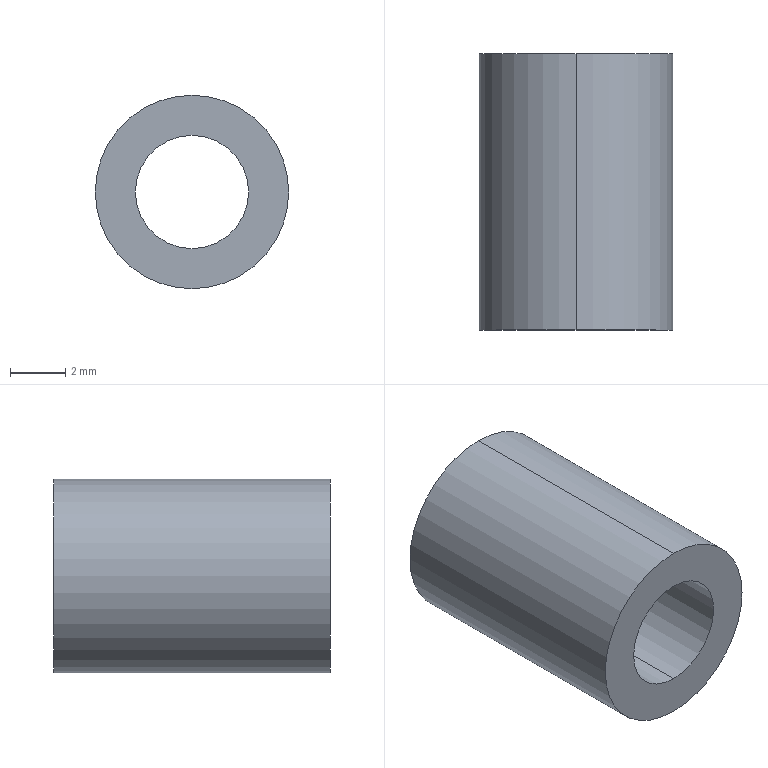Part | SolidWorks | features BaseBody 1 | 1 solid | 6 faces | box 7 x 10 x 7 mm | volume 252.82 mm3 | cylinder 4 | plane 2 | commonest cylinder face diameters 4.1 x2 7 x2
STEP:
#1=CARTESIAN_POINT('',(0.,5.,-3.5));
#2=VERTEX_POINT('',#1);
#3=CARTESIAN_POINT('',(0.,5.,3.5));
#4=VERTEX_POINT('',#3);
#5=CARTESIAN_POINT('',(0.,5.,0.));
#6=DIRECTION('',(0.,-1.,0.));
#7=DIRECTION('',(0.,0.,-1.));
#8=AXIS2_PLACEMENT_3D('',#5,#6,#7);
#9=CIRCLE('',#8,3.5);
#10=EDGE_CURVE('',#2,#4,#9,.T.);
#11=ORIENTED_EDGE('',*,*,#10,.T.);
#12=CARTESIAN_POINT('',(0.,-5.,3.5));
#13=VERTEX_POINT('',#12);
#14=CARTESIAN_POINT('',(0.,5.,3.5));
#15=DIRECTION('',(0.,-1.,0.));
#16=VECTOR('',#15,1000.);
#17=LINE('',#14,#16);
#18=EDGE_CURVE('',#4,#13,#17,.T.);
#19=ORIENTED_EDGE('',*,*,#18,.T.);
#20=CARTESIAN_POINT('',(0.,-5.,-3.5));
#21=VERTEX_POINT('',#20);
#22=CARTESIAN_POINT('',(0.,-5.,0.));
#23=DIRECTION('',(0.,1.,0.));
#24=DIRECTION('',(0.,0.,-1.));
#25=AXIS2_PLACEMENT_3D('',#22,#23,#24);
#26=CIRCLE('',#25,3.5);
#27=EDGE_CURVE('',#13,#21,#26,.T.);
#28=ORIENTED_EDGE('',*,*,#27,.T.);
#29=CARTESIAN_POINT('',(0.,5.,-3.5));
#30=DIRECTION('',(0.,-1.,0.));
#31=VECTOR('',#30,1000.);
#32=LINE('',#29,#31);
#33=EDGE_CURVE('',#2,#21,#32,.T.);
#34=ORIENTED_EDGE('',*,*,#33,.F.);
#35=EDGE_LOOP('',(#11,#19,#28,#34));
#36=FACE_OUTER_BOUND('',#35,.T.);
#37=CARTESIAN_POINT('',(0.,5.,0.));
#38=DIRECTION('',(0.,-1.,0.));
#39=DIRECTION('',(0.,0.,-1.));
#40=AXIS2_PLACEMENT_3D('',#37,#38,#39);
#41=CYLINDRICAL_SURFACE('',#40,3.5);
#42=ADVANCED_FACE('',(#36),#41,.T.);
#43=CARTESIAN_POINT('',(0.,5.,2.05));
#44=VERTEX_POINT('',#43);
#45=CARTESIAN_POINT('',(0.,5.,-2.05));
#46=VERTEX_POINT('',#45);
#47=CARTESIAN_POINT('',(0.,5.,0.));
#48=DIRECTION('',(0.,-1.,0.));
#49=DIRECTION('',(0.,0.,-1.));
#50=AXIS2_PLACEMENT_3D('',#47,#48,#49);
#51=CIRCLE('',#50,2.05);
#52=EDGE_CURVE('',#44,#46,#51,.T.);
#53=ORIENTED_EDGE('',*,*,#52,.F.);
#54=CARTESIAN_POINT('',(0.,-5.,2.05));
#55=VERTEX_POINT('',#54);
#56=CARTESIAN_POINT('',(0.,5.,2.05));
#57=DIRECTION('',(0.,-1.,0.));
#58=VECTOR('',#57,1000.);
#59=LINE('',#56,#58);
#60=EDGE_CURVE('',#44,#55,#59,.T.);
#61=ORIENTED_EDGE('',*,*,#60,.T.);
#62=CARTESIAN_POINT('',(0.,-5.,-2.05));
#63=VERTEX_POINT('',#62);
#64=CARTESIAN_POINT('',(0.,-5.,0.));
#65=DIRECTION('',(0.,-1.,0.));
#66=DIRECTION('',(0.,0.,-1.));
#67=AXIS2_PLACEMENT_3D('',#64,#65,#66);
#68=CIRCLE('',#67,2.05);
#69=EDGE_CURVE('',#55,#63,#68,.T.);
#70=ORIENTED_EDGE('',*,*,#69,.T.);
#71=CARTESIAN_POINT('',(0.,5.,-2.05));
#72=DIRECTION('',(0.,-1.,0.));
#73=VECTOR('',#72,1000.);
#74=LINE('',#71,#73);
#75=EDGE_CURVE('',#46,#63,#74,.T.);
#76=ORIENTED_EDGE('',*,*,#75,.F.);
#77=EDGE_LOOP('',(#53,#61,#70,#76));
#78=FACE_OUTER_BOUND('',#77,.T.);
#79=CARTESIAN_POINT('',(0.,5.,0.));
#80=DIRECTION('',(0.,-1.,0.));
#81=DIRECTION('',(0.,0.,-1.));
#82=AXIS2_PLACEMENT_3D('',#79,#80,#81);
#83=CYLINDRICAL_SURFACE('',#82,2.05);
#84=ADVANCED_FACE('',(#78),#83,.F.);
#85=ORIENTED_EDGE('',*,*,#18,.F.);
#86=CARTESIAN_POINT('',(0.,5.,0.));
#87=DIRECTION('',(0.,-1.,0.));
#88=DIRECTION('',(0.,0.,-1.));
#89=AXIS2_PLACEMENT_3D('',#86,#87,#88);
#90=CIRCLE('',#89,3.5);
#91=EDGE_CURVE('',#4,#2,#90,.T.);
#92=ORIENTED_EDGE('',*,*,#91,.T.);
#93=ORIENTED_EDGE('',*,*,#33,.T.);
#94=CARTESIAN_POINT('',(0.,-5.,0.));
#95=DIRECTION('',(0.,1.,0.));
#96=DIRECTION('',(0.,0.,-1.));
#97=AXIS2_PLACEMENT_3D('',#94,#95,#96);
#98=CIRCLE('',#97,3.5);
#99=EDGE_CURVE('',#21,#13,#98,.T.);
#100=ORIENTED_EDGE('',*,*,#99,.T.);
#101=EDGE_LOOP('',(#85,#92,#93,#100));
#102=FACE_OUTER_BOUND('',#101,.T.);
#103=CARTESIAN_POINT('',(0.,5.,0.));
#104=DIRECTION('',(0.,-1.,0.));
#105=DIRECTION('',(0.,0.,-1.));
#106=AXIS2_PLACEMENT_3D('',#103,#104,#105);
#107=CYLINDRICAL_SURFACE('',#106,3.5);
#108=ADVANCED_FACE('',(#102),#107,.T.);
#109=CARTESIAN_POINT('',(0.,-5.,0.));
#110=DIRECTION('',(0.,-1.,0.));
#111=DIRECTION('',(0.,0.,-1.));
#112=AXIS2_PLACEMENT_3D('',#109,#110,#111);
#113=CIRCLE('',#112,2.05);
#114=EDGE_CURVE('',#63,#55,#113,.T.);
#115=ORIENTED_EDGE('',*,*,#114,.F.);
#116=ORIENTED_EDGE('',*,*,#69,.F.);
#117=EDGE_LOOP('',(#115,#116));
#118=FACE_BOUND('',#117,.T.);
#119=ORIENTED_EDGE('',*,*,#99,.F.);
#120=ORIENTED_EDGE('',*,*,#27,.F.);
#121=EDGE_LOOP('',(#119,#120));
#122=FACE_OUTER_BOUND('',#121,.T.);
#123=CARTESIAN_POINT('',(0.,-5.,0.));
#124=DIRECTION('',(0.,1.,0.));
#125=DIRECTION('',(0.,0.,1.));
#126=AXIS2_PLACEMENT_3D('',#123,#124,#125);
#127=PLANE('',#126);
#128=ADVANCED_FACE('',(#118,#122),#127,.F.);
#129=CARTESIAN_POINT('',(0.,5.,0.));
#130=DIRECTION('',(0.,-1.,0.));
#131=DIRECTION('',(0.,0.,-1.));
#132=AXIS2_PLACEMENT_3D('',#129,#130,#131);
#133=CIRCLE('',#132,2.05);
#134=EDGE_CURVE('',#46,#44,#133,.T.);
#135=ORIENTED_EDGE('',*,*,#134,.T.);
#136=ORIENTED_EDGE('',*,*,#52,.T.);
#137=EDGE_LOOP('',(#135,#136));
#138=FACE_BOUND('',#137,.T.);
#139=ORIENTED_EDGE('',*,*,#10,.F.);
#140=ORIENTED_EDGE('',*,*,#91,.F.);
#141=EDGE_LOOP('',(#139,#140));
#142=FACE_OUTER_BOUND('',#141,.T.);
#143=CARTESIAN_POINT('',(0.,5.,0.));
#144=DIRECTION('',(0.,1.,0.));
#145=DIRECTION('',(0.,0.,1.));
#146=AXIS2_PLACEMENT_3D('',#143,#144,#145);
#147=PLANE('',#146);
#148=ADVANCED_FACE('',(#138,#142),#147,.T.);
#149=ORIENTED_EDGE('',*,*,#60,.F.);
#150=ORIENTED_EDGE('',*,*,#134,.F.);
#151=ORIENTED_EDGE('',*,*,#75,.T.);
#152=ORIENTED_EDGE('',*,*,#114,.T.);
#153=EDGE_LOOP('',(#149,#150,#151,#152));
#154=FACE_OUTER_BOUND('',#153,.T.);
#155=CARTESIAN_POINT('',(0.,5.,0.));
#156=DIRECTION('',(0.,-1.,0.));
#157=DIRECTION('',(0.,0.,-1.));
#158=AXIS2_PLACEMENT_3D('',#155,#156,#157);
#159=CYLINDRICAL_SURFACE('',#158,2.05);
#160=ADVANCED_FACE('',(#154),#159,.F.);
#161=CLOSED_SHELL('',(#42,#84,#108,#128,#148,#160));
#162=MANIFOLD_SOLID_BREP('',#161);
#163=CARTESIAN_POINT('',(0.,0.,0.));
#164=DIRECTION('',(0.,0.,1.));
#165=DIRECTION('',(1.,0.,0.));
#166=AXIS2_PLACEMENT_3D('',#163,#164,#165);
#167=(LENGTH_UNIT()NAMED_UNIT(*)SI_UNIT(.MILLI.,.METRE.));
#168=UNCERTAINTY_MEASURE_WITH_UNIT(LENGTH_MEASURE(0.00001),#167,'','');
#169=(NAMED_UNIT(*)PLANE_ANGLE_UNIT()SI_UNIT($,.RADIAN.));
#170=(NAMED_UNIT(*)SI_UNIT($,.STERADIAN.)SOLID_ANGLE_UNIT());
#171=(GEOMETRIC_REPRESENTATION_CONTEXT(3)GLOBAL_UNCERTAINTY_ASSIGNED_CONTEXT((#168))GLOBAL_UNIT_ASSIGNED_CONTEXT((#167,#169,#170))REPRESENTATION_CONTEXT('',''));
#172=ADVANCED_BREP_SHAPE_REPRESENTATION('',(#162,#166),#171);